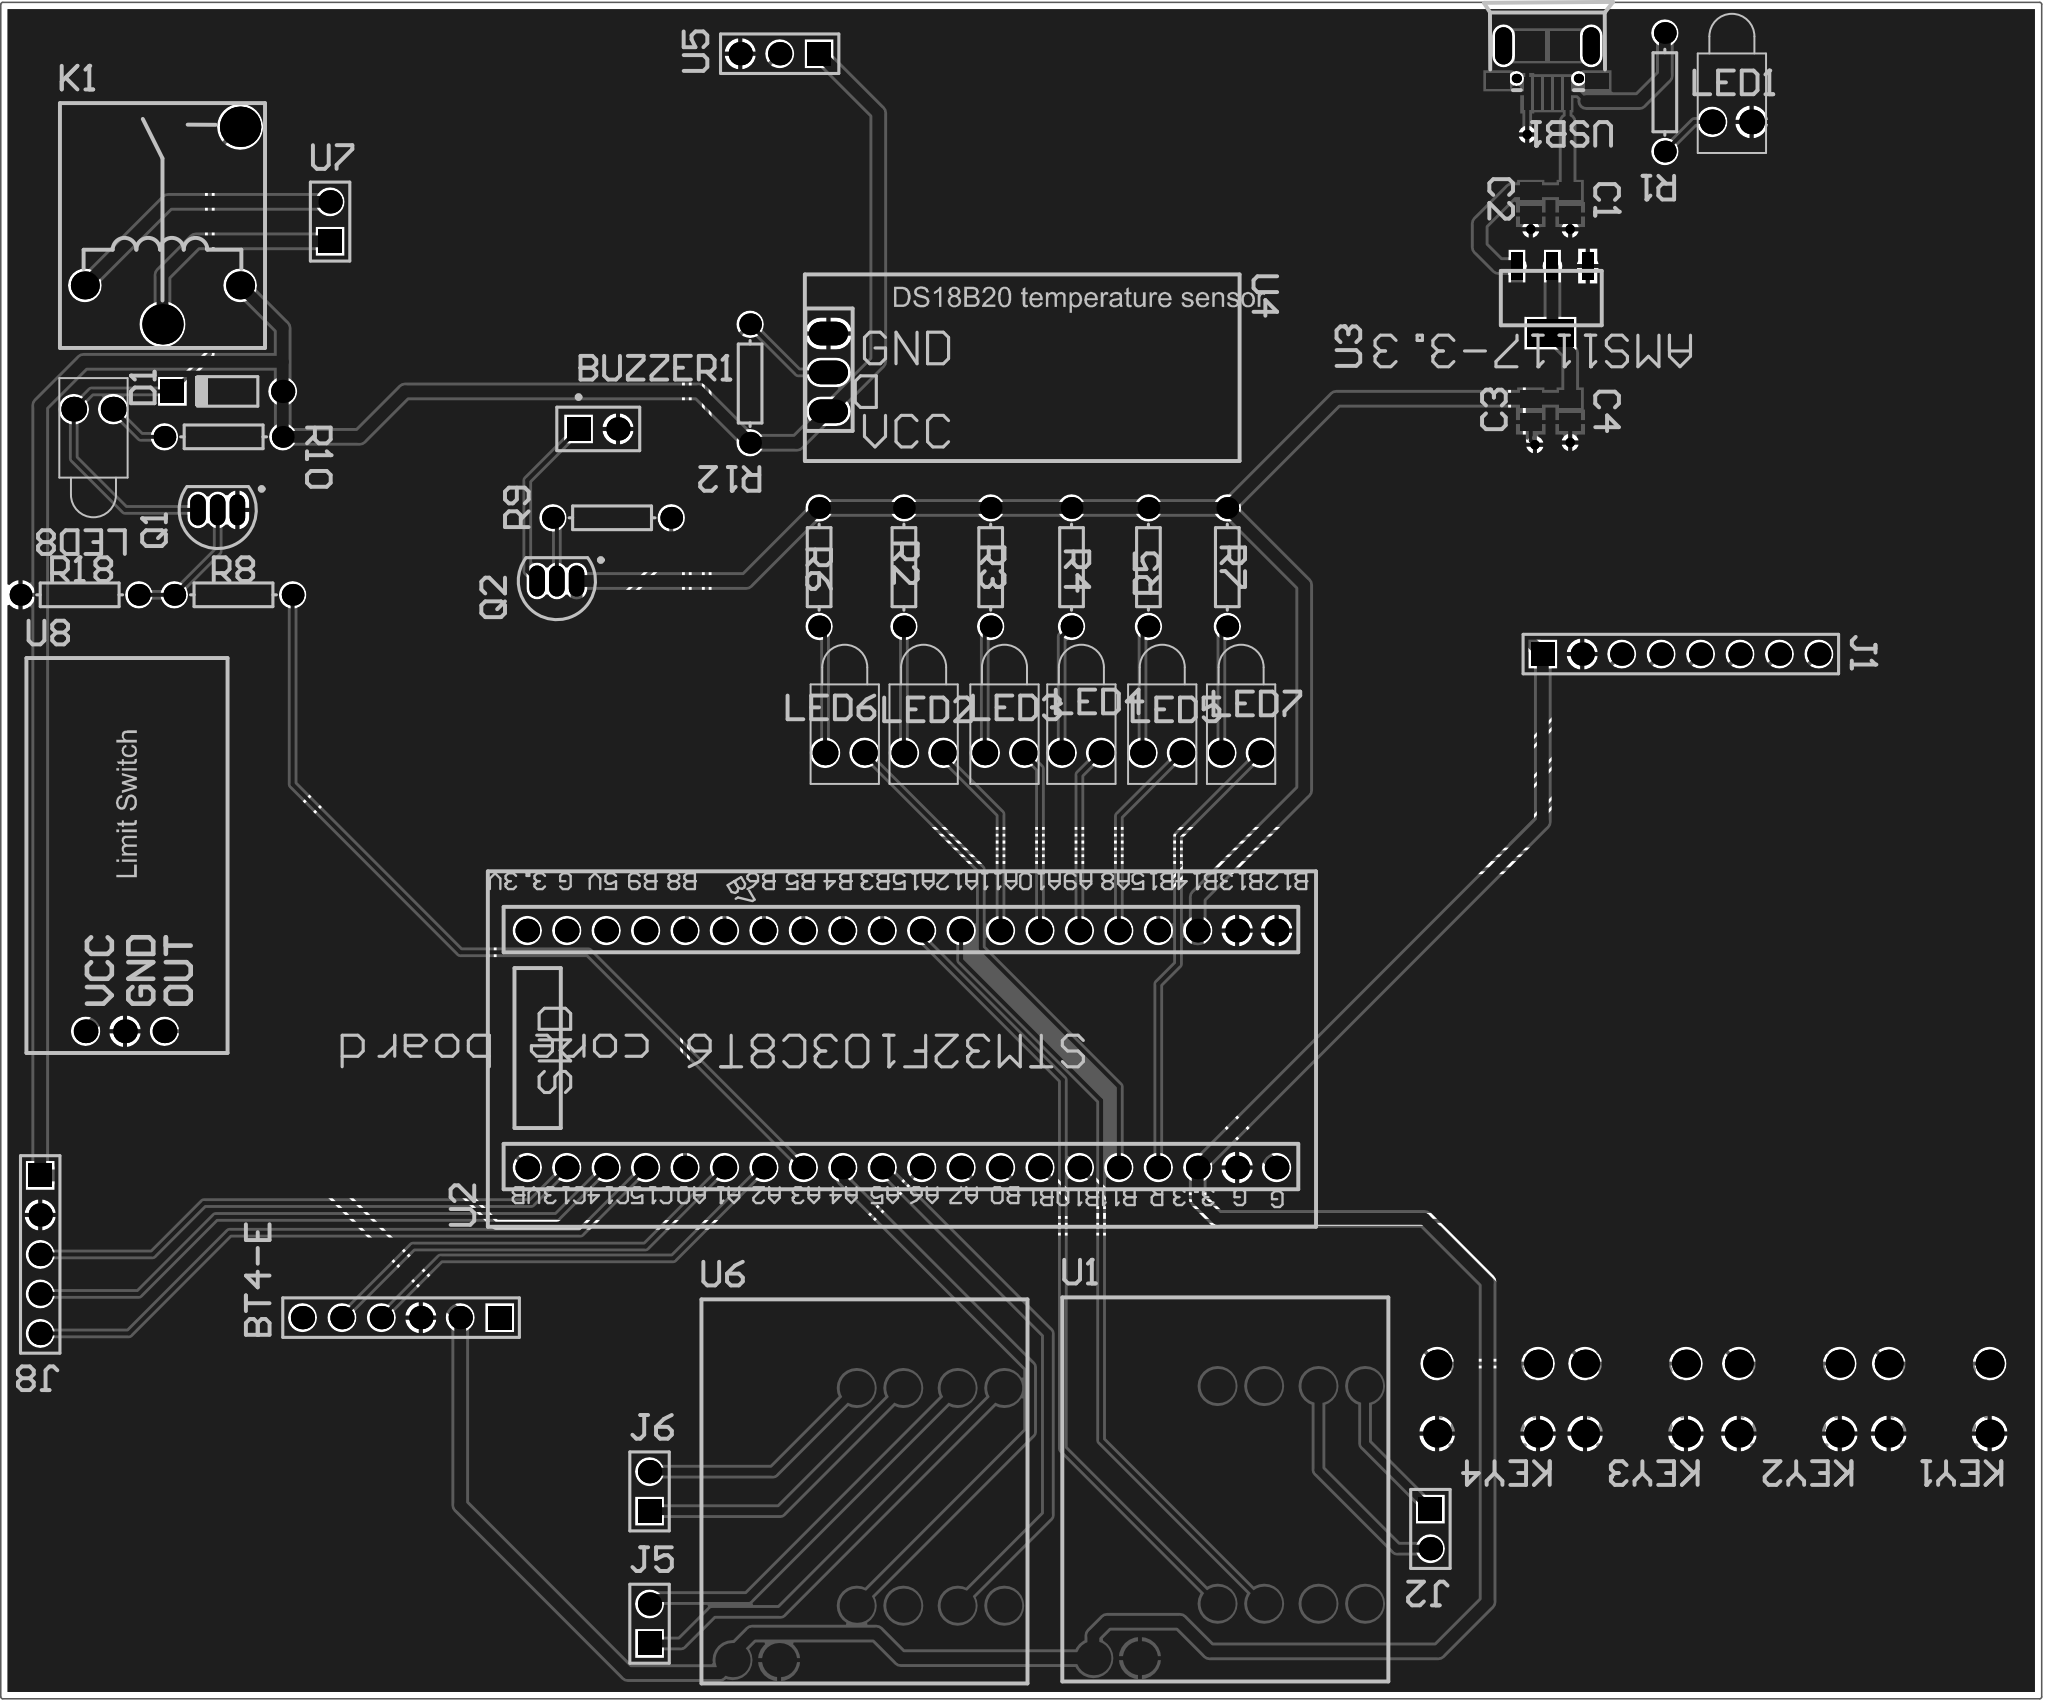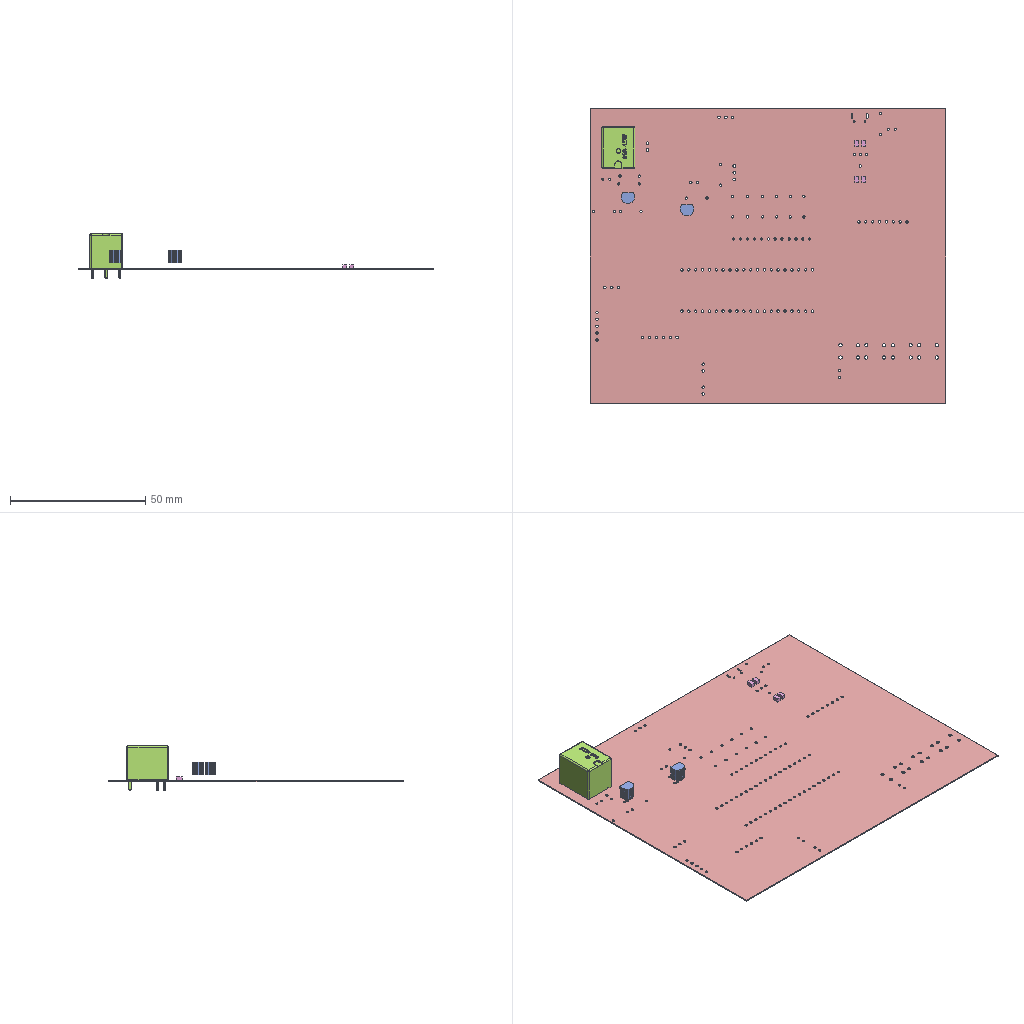Circuit board layout | Altium Designer | box 131.4 x 109.1 x 16.5 mm
Layer stack:
# Altium Designer layer stack of  (unit mm; dielectric type: 0 none, 1 core, 2 prepreg, 3 surface material)
index,name,kind,layer,copper_thickness_mm,dielectric_type,dielectric_thickness_mm,dielectric_material,dielectric_constant
0,Top Paste,other,,,,,,
1,Top Overlay,other,,,,,,
2,Top Solder,dielectric,,,3,0.0102,Solder Resist,3.5
3,Top Layer,copper,Top Layer,0.0356,,,,
4,Dielectric 1,dielectric,,,0,0.32,FR-4,4.8
5,Bottom Layer,copper,Bottom Layer,0.0356,,,,
6,Bottom Solder,dielectric,,,3,0.0102,Solder Resist,3.5
7,Bottom Overlay,other,,,,,,
8,Bottom Paste,other,,,,,,
# drill layer pairs: low layer,high layer
drill_pair,Top Layer,Bottom Layer
Part placement:
Designator,Comment,Layer,Footprint,Center-X(mm),Center-Y(mm),Rotation
USB1,MICRO5.9MMUSB,TopLayer,MICRO-USB-SMD_5P-P0.65-H-F_MICRO5.9MMUSB,124.884,122.808,180
U8,NO,TopLayer,xianwei,33.274,60.96,90
U7,Connect watering pump,TopLayer,HDR1X2,46.482,113.03,90
U6,1508S motor driver module,TopLayer,DIANJIQUDONG,81.149,29.269,90
U5,NO,TopLayer,HDR1X3,75.438,123.825,180
U4,DS18B20,TopLayer,DS18B20,78.579,103.33,360
U3,AMS1117-3.3,TopLayer,AMS1117-3.3,125.202,108.011,180
U2,STM32F103C8T6 core board,TopLayer,STM32核心板,83.312,59.817,90
U1,1508S motor driver module,TopLayer,DIANJIQUDONG,104.39,29.396,90
R18,10k,TopLayer,AXIAL-0.3,30.353,89.027,360
R12,4.7k,TopLayer,AXIAL-0.3,73.533,102.616,270
R10,4.7K,TopLayer,AXIAL-0.3,39.624,99.187,360
R9,1k,TopLayer,AXIAL-0.3,64.643,93.98,180
R8,1k,TopLayer,AXIAL-0.3,40.259,89.027,180
R7,1k,TopLayer,AXIAL-0.3,104.267,90.805,270
R6,1k,TopLayer,AXIAL-0.3,77.978,90.805,270
R5,1k,TopLayer,AXIAL-0.3,99.187,90.805,270
R4,1k,TopLayer,AXIAL-0.3,94.234,90.805,270
R3,1k,TopLayer,AXIAL-0.3,89.027,90.805,270
R2,1k,TopLayer,AXIAL-0.3,83.439,90.805,270
R1,4.7k,TopLayer,AXIAL-0.3,132.447,121.346,270
Q2,S8550,TopLayer,TO-92A,61.087,89.916,90
Q1,S8050-D,TopLayer,TO-92A,39.243,94.488,90
LED8,LED-TH-3mm_R,TopLayer,LED-1,31.242,100.965,270
LED7,LED-0603_R,TopLayer,LED-1,105.156,78.867,90
LED6,LED-0603_R,TopLayer,LED-1,79.629,78.867,90
LED5,LED-0603_R,TopLayer,LED-1,100.076,78.867,90
LED4,LED-0603_R,TopLayer,LED-1,94.869,78.867,90
LED3,LED-0603_R,TopLayer,LED-1,89.916,78.867,90
LED2,LED-0603_R,TopLayer,LED-1,84.709,78.867,90
LED1,LED-TH-3mm_R,TopLayer,LED-1,136.765,119.441,90
KEY4,K4-6×6_TH,TopLayer,四脚轻触开关,121.031,37.338,180
KEY3,K4-6×6_TH,TopLayer,四脚轻触开关,130.556,37.338,180
KEY2,K4-6×6_TH,TopLayer,四脚轻触开关,140.462,37.338,180
KEY1,K4-6×6_TH,TopLayer,四脚轻触开关,150.114,37.338,180
K1,SRD-5VDC-SL-A,TopLayer,012-1HW_BK,35.687,112.776,90
J8,HDR-M-2.54_1x5,TopLayer,HDR1X5,27.813,46.609,270
J6,HDR-M-2.54_1x2,TopLayer,HDR1X2,67.056,31.369,90
J5,HDR-M-2.54_1x2,TopLayer,HDR1X2,67.056,22.86,90
J2,HDR-M-2.54_1x2,TopLayer,HDR1X2,117.348,28.956,270
J1,HDR-M-2.54_1x8,TopLayer,HDR1X8,133.477,85.217,360
D1,1N4148,TopLayer,DO-35,39.878,102.108,180
C4,100nF,TopLayer,C0805,126.351,100.887,270
C3,10uF,TopLayer,C0805,123.811,100.887,90
C2,100nF,TopLayer,C0805,123.811,114.234,270
C1,10uF,TopLayer,C0805,126.351,114.234,270
BUZZER1,5V,TopLayer,PIN2,63.754,99.695,360
BT4-E,NO,TopLayer,HDR1X6,51.054,42.545,180
Pad and via stacks:
# Altium Designer via and pad stacks of  (unit mm). Each distinct definition once, with the count of objects using it.
# via: kind,start_layer,end_layer,hole_mm,diameter_mm,mode(0 simple;1 top-mid-bottom;2 full stack),diameter_per_layer,count,example_net
# pad: kind,layer,hole_mm,hole_type(0 round;1 square;2 slot),plating,top_size,top_shape(1 round;2 rect;3 octagon;9 rounded rect),mid_size,bottom_size,mode,footprint,size_per_layer,count,example
pad,Multi-Layer,0.9144,2,plated,1.524x1.524,1,1.524x1.524,1.524x1.524,0,STM32\u00BA\u00CB\u00D0\u00C4\u00B0\u00E5,,40,U2.1
pad,Multi-Layer,0.85,0,plated,1.4x1.4,1,1.4x1.4,1.4x1.4,0,AXIAL-0.3,,24,R1.2
pad,Multi-Layer,0.6,2,plated,1.1x2.4,1,1.1x2.4,1.1x2.4,0,MICRO-USB-SMD_5P-P0.65-H-F_MICRO5.9MMUSB,,2,USB1.6
pad,Multi-Layer,0.6,0,unplated,0.6x0.6,1,0.6x0.6,0.6x0.6,0,MICRO-USB-SMD_5P-P0.65-H-F_MICRO5.9MMUSB,,2,USB1.
pad,Multi-Layer,0.8,0,plated,1.6x1.6,1,1.6x1.6,1.6x1.6,0,LED-1,,16,LED1.1
pad,Multi-Layer,0.9,2,plated,2.524x1.524,1,2.524x1.524,2.524x1.524,0,DS18B20,,3,U4.2
pad,Multi-Layer,0.9,0,plated,1.5x1.5,2,1.5x1.5,1.5x1.5,0,HDR1X6,,1,BT4-E.1
pad,Multi-Layer,0.9,0,plated,1.5x1.5,1,1.5x1.5,1.5x1.5,0,HDR1X6,,5,BT4-E.2
pad,Multi-Layer,0.9144,0,plated,3x1.75,2,3x1.75,3x1.75,0,AMS1117-3.3,,1,U3.4
pad,Multi-Layer,0.9144,0,plated,0.74x1.75,2,0.74x1.75,0.74x1.75,0,AMS1117-3.3,,3,U3.3
pad,Multi-Layer,0.9,0,plated,1.5x1.5,2,1.5x1.5,1.5x1.5,0,HDR1X2,,4,J2.1
pad,Multi-Layer,0.9,0,plated,1.5x1.5,1,1.5x1.5,1.5x1.5,0,HDR1X2,,4,J2.2
pad,Multi-Layer,0.9,0,plated,1.5x1.5,2,1.5x1.5,1.5x1.5,0,PIN2,,1,BUZZER1.1
pad,Multi-Layer,0.9,0,plated,1.5x1.5,1,1.5x1.5,1.5x1.5,0,PIN2,,1,BUZZER1.2
pad,Multi-Layer,0.9,0,plated,2x1,1,2x1,2x1,0,TO-92A,,6,Q2.3
pad,Multi-Layer,0.9,0,plated,1.5x1.5,1,1.5x1.5,1.5x1.5,0,HDR1X5,,4,J8.5
pad,Multi-Layer,0.9,0,plated,1.5x1.5,2,1.5x1.5,1.5x1.5,0,HDR1X5,,1,J8.1
pad,Multi-Layer,0.9,0,plated,1.5x1.5,2,1.5x1.5,1.5x1.5,0,HDR1X3,,1,U5.1
pad,Multi-Layer,0.9,0,plated,1.5x1.5,1,1.5x1.5,1.5x1.5,0,HDR1X3,,2,U5.2
pad,Multi-Layer,1.6,0,plated,2.6x2.6,1,2.6x2.6,2.6x2.6,0,012-1HW_BK,,2,K1.4
pad,Multi-Layer,1,0,plated,1.8x1.8,1,1.8x1.8,1.8x1.8,0,012-1HW_BK,,2,K1.2
pad,Multi-Layer,1.2,0,plated,1.8x1.8,1,1.8x1.8,1.8x1.8,0,\u00CB\u00C4\u00BD\u00C5\u00C7\u00E1\u00B4\u00A5\u00BF\u00AA\u00B9\u00D8,,16,KEY1.4
pad,Multi-Layer,0.9,0,plated,1.5x1.5,2,1.5x1.5,1.5x1.5,0,DO-35,,1,D1.2
pad,Multi-Layer,0.9,0,plated,1.5x1.5,1,1.5x1.5,1.5x1.5,0,DO-35,,1,D1.1
pad,Multi-Layer,0.9,0,plated,1.5x1.5,2,1.5x1.5,1.5x1.5,0,HDR1X8,,1,J1.1
pad,Multi-Layer,0.9,0,plated,1.5x1.5,1,1.5x1.5,1.5x1.5,0,HDR1X8,,7,J1.2
pad,Multi-Layer,0.9144,0,plated,1.524x1.524,1,1.524x1.524,1.524x1.524,0,xianwei,,3,U8.3
pad,Top Layer,0,0,plated,1.9x1.9,2,1.9x1.9,1.9x1.9,0,MICRO-USB-SMD_5P-P0.65-H-F_MICRO5.9MMUSB,,2,USB1.6
pad,Top Layer,0,0,plated,1.5x1,2,1.5x1,1.5x1,0,MICRO-USB-SMD_5P-P0.65-H-F_MICRO5.9MMUSB,,2,USB1.6
pad,Top Layer,0,0,plated,0.4x2.1,2,0.4x2.1,0.4x2.1,0,MICRO-USB-SMD_5P-P0.65-H-F_MICRO5.9MMUSB,,5,USB1.5
pad,Top Layer,0,0,plated,1.4x1.1,2,1.4x1.1,1.4x1.1,0,C0805,,8,C4.2
pad,Top Layer,0,0,plated,2.2x2.2,1,2.2x2.2,2.2x2.2,0,DIANJIQUDONG,,20,U1.3
via,Top Layer,Bottom Layer,0.3048,0.6096,0,,5,GND
Copper pours:
name,layer,net,type(0 solid;1 hatched;2 none)
G,Top Layer,GND,0
G,Bottom Layer,GND,0
Design rules, without the lines most boards share:
# Altium Designer design rules of  (exported by Altium Designer, unit mm)
# columns: name | kind | enabled | priority | scope1 | scope2 | descriptor | typed fields (field=value)
Clearance | 0 | enabled | 1 | All | All | Clearance Constraint (Gap=7mil) (All),(All) | gap=0.1778
PlaneConnect | 6 | enabled | 1 | All | All | Power Plane Connect Rule(Relief Connect )(Expansion=20mil) (Conductor Width=10mil) (Air Gap=10mil) (Entries=4) (All) | relief_conductor_width=0.254 relief_entries=4 relief_expansion=0.508
PolygonConnect | 20 | enabled | 1 | All | All | Polygon Connect Rule(Relief Connect )(Conductor Width=10mil) (Relief Angle=90 Angle) (Entries=4) (Air Gap Width=10mil) (All),(All) | connect_style(0=relief,1=direct,2=none)=0 relief_conductor_width=0.254 relief_entries=4
Width | 2 | enabled | 1 | All | All | Width Constraint (Min=10mil) (Max=30mil) (Preferred=10mil) (All) |
RoutingVias | 11 | enabled | 1 | All | All | Routing Via (MinHoleWidth=28mil) (MaxHoleWidth=28mil) (PreferredHoleWidth=28mil) (MinWidth=50mil) (MaxWidth=50mil) (PreferedWidth=50mil) (All) | via_min_hole=0.7112 via_max_hole=0.7112 via_preferred_diameter=1.27 via_preferred_hole=0.7112
PasteMaskExpansion | 14 | enabled | 1 | All | All | Paste Mask Expansion (Expansion =0mil) (All) | expansion=0
SolderMaskExpansion | 13 | enabled | 1 | All | All | Solder Mask Expansion (Expansion =4mil) (All) | expansion=0.1016
DiffPairsRouting | 51 | enabled | 1 | All | All | Differential Pairs Uncoupled Length using the Gap Constraints (Min=10mil) (Max=10mil) (Prefered=10mil)  and Width Constraints (Min=15mil) (Max=15mil) (Prefered=15mil) (All) |
HoleToHoleClearance | 52 | enabled | 1 | All | All | Hole To Hole Clearance (Gap=10mil) (All),(All) | gap=0.254
MinimumSolderMaskSliver | 53 | enabled | 1 | All | All | Minimum Solder Mask Sliver (Gap=0mil) (All),(All) |
SilkToSolderMaskClearance | 54 | enabled | 1 | IsPad | All | Silk To Solder Mask (Clearance=0mil) (IsPad),(All) |
SilkToSilkClearance | 55 | enabled | 1 | All | All | Silk to Silk (Clearance=0mil) (All),(All) |